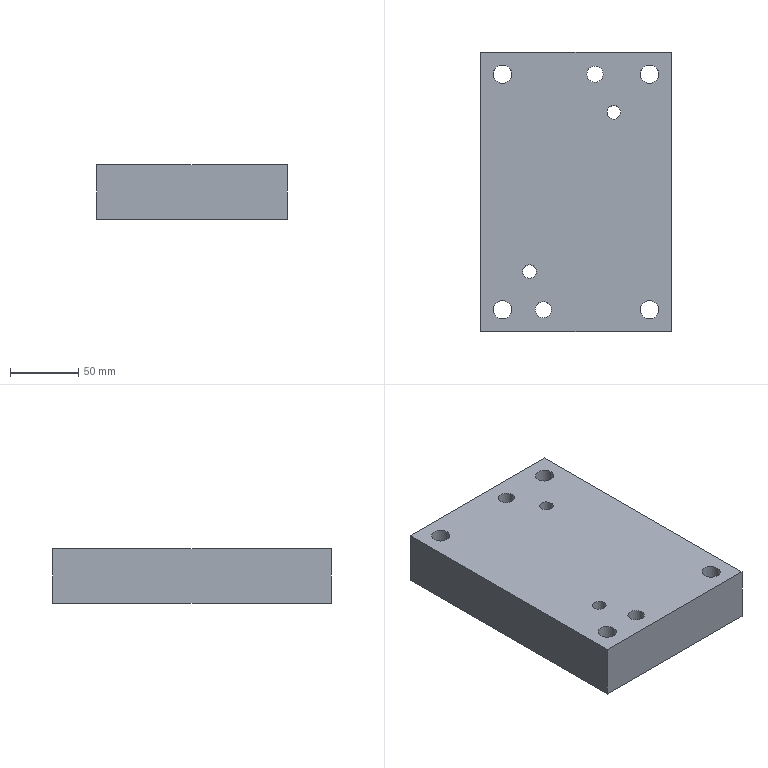Part | STEP file | lll_id762_x_t | 1 solid | 36 faces | box 140 x 205 x 40 mm | volume 1088950 mm3 | cylinder 19 | plane 10 | cone 7 | commonest cylinder face diameters 8.506 x4 13.509 x4 20.007 x4 8.505 x3 10 x2 12 x2
STEP:
#1=CARTESIAN_POINT('',(3881.234,-22.52,102.5));
#2=VERTEX_POINT('',#1);
#3=CARTESIAN_POINT('',(3876.982,-22.52,102.5));
#4=DIRECTION('',(0.,0.,1.));
#5=DIRECTION('',(1.,0.,0.));
#6=AXIS2_PLACEMENT_3D('',#3,#4,#5);
#7=CIRCLE('',#6,4.253);
#8=EDGE_CURVE('',#2,#2,#7,.T.);
#9=ORIENTED_EDGE('',*,*,#8,.T.);
#10=EDGE_LOOP('',(#9));
#11=FACE_BOUND('',#10,.T.);
#12=CARTESIAN_POINT('',(3798.187,86.5,102.5));
#13=VERTEX_POINT('',#12);
#14=CARTESIAN_POINT('',(3788.184,86.5,102.5));
#15=DIRECTION('',(0.,0.,1.));
#16=DIRECTION('',(1.,0.,0.));
#17=AXIS2_PLACEMENT_3D('',#14,#15,#16);
#18=CIRCLE('',#17,10.004);
#19=EDGE_CURVE('',#13,#13,#18,.T.);
#20=ORIENTED_EDGE('',*,*,#19,.T.);
#21=EDGE_LOOP('',(#20));
#22=FACE_BOUND('',#21,.T.);
#23=CARTESIAN_POINT('',(3798.187,-86.5,102.5));
#24=VERTEX_POINT('',#23);
#25=CARTESIAN_POINT('',(3788.184,-86.5,102.5));
#26=DIRECTION('',(0.,0.,1.));
#27=DIRECTION('',(1.,0.,0.));
#28=AXIS2_PLACEMENT_3D('',#25,#26,#27);
#29=CIRCLE('',#28,10.004);
#30=EDGE_CURVE('',#24,#24,#29,.T.);
#31=ORIENTED_EDGE('',*,*,#30,.T.);
#32=EDGE_LOOP('',(#31));
#33=FACE_BOUND('',#32,.T.);
#34=CARTESIAN_POINT('',(3812.184,-86.5,102.5));
#35=VERTEX_POINT('',#34);
#36=CARTESIAN_POINT('',(3818.184,-86.5,102.5));
#37=DIRECTION('',(0.,0.,-1.));
#38=DIRECTION('',(-1.,0.,0.));
#39=AXIS2_PLACEMENT_3D('',#36,#37,#38);
#40=CIRCLE('',#39,6.);
#41=EDGE_CURVE('',#35,#35,#40,.T.);
#42=ORIENTED_EDGE('',*,*,#41,.F.);
#43=EDGE_LOOP('',(#42));
#44=FACE_BOUND('',#43,.T.);
#45=CARTESIAN_POINT('',(3890.747,58.5,102.5));
#46=VERTEX_POINT('',#45);
#47=CARTESIAN_POINT('',(3895.,58.5,102.5));
#48=DIRECTION('',(0.,0.,-1.));
#49=DIRECTION('',(-1.,0.,0.));
#50=AXIS2_PLACEMENT_3D('',#47,#48,#49);
#51=CIRCLE('',#50,4.253);
#52=EDGE_CURVE('',#46,#46,#51,.T.);
#53=ORIENTED_EDGE('',*,*,#52,.F.);
#54=EDGE_LOOP('',(#53));
#55=FACE_BOUND('',#54,.T.);
#56=CARTESIAN_POINT('',(3785.747,-58.5,102.5));
#57=VERTEX_POINT('',#56);
#58=CARTESIAN_POINT('',(3790.,-58.5,102.5));
#59=DIRECTION('',(0.,0.,-1.));
#60=DIRECTION('',(-1.,0.,0.));
#61=AXIS2_PLACEMENT_3D('',#58,#59,#60);
#62=CIRCLE('',#61,4.253);
#63=EDGE_CURVE('',#57,#57,#62,.T.);
#64=ORIENTED_EDGE('',*,*,#63,.F.);
#65=EDGE_LOOP('',(#64));
#66=FACE_BOUND('',#65,.T.);
#67=CARTESIAN_POINT('',(3795.747,58.5,102.5));
#68=VERTEX_POINT('',#67);
#69=CARTESIAN_POINT('',(3800.,58.5,102.5));
#70=DIRECTION('',(0.,0.,-1.));
#71=DIRECTION('',(-1.,0.,0.));
#72=AXIS2_PLACEMENT_3D('',#69,#70,#71);
#73=CIRCLE('',#72,4.253);
#74=EDGE_CURVE('',#68,#68,#73,.T.);
#75=ORIENTED_EDGE('',*,*,#74,.F.);
#76=EDGE_LOOP('',(#75));
#77=FACE_BOUND('',#76,.T.);
#78=CARTESIAN_POINT('',(3890.747,-58.5,102.5));
#79=VERTEX_POINT('',#78);
#80=CARTESIAN_POINT('',(3895.,-58.5,102.5));
#81=DIRECTION('',(0.,0.,-1.));
#82=DIRECTION('',(-1.,0.,0.));
#83=AXIS2_PLACEMENT_3D('',#80,#81,#82);
#84=CIRCLE('',#83,4.253);
#85=EDGE_CURVE('',#79,#79,#84,.T.);
#86=ORIENTED_EDGE('',*,*,#85,.F.);
#87=EDGE_LOOP('',(#86));
#88=FACE_BOUND('',#87,.T.);
#89=CARTESIAN_POINT('',(3803.,-58.5,102.5));
#90=VERTEX_POINT('',#89);
#91=CARTESIAN_POINT('',(3808.,-58.5,102.5));
#92=DIRECTION('',(0.,0.,-1.));
#93=DIRECTION('',(-1.,0.,0.));
#94=AXIS2_PLACEMENT_3D('',#91,#92,#93);
#95=CIRCLE('',#94,5.);
#96=EDGE_CURVE('',#90,#90,#95,.T.);
#97=ORIENTED_EDGE('',*,*,#96,.F.);
#98=EDGE_LOOP('',(#97));
#99=FACE_BOUND('',#98,.T.);
#100=CARTESIAN_POINT('',(3865.,58.5,102.5));
#101=VERTEX_POINT('',#100);
#102=CARTESIAN_POINT('',(3870.,58.5,102.5));
#103=DIRECTION('',(0.,0.,-1.));
#104=DIRECTION('',(-1.,0.,0.));
#105=AXIS2_PLACEMENT_3D('',#102,#103,#104);
#106=CIRCLE('',#105,5.);
#107=EDGE_CURVE('',#101,#101,#106,.T.);
#108=ORIENTED_EDGE('',*,*,#107,.F.);
#109=EDGE_LOOP('',(#108));
#110=FACE_BOUND('',#109,.T.);
#111=CARTESIAN_POINT('',(3772.184,102.5,102.5));
#112=VERTEX_POINT('',#111);
#113=CARTESIAN_POINT('',(3772.184,-102.5,102.5));
#114=VERTEX_POINT('',#113);
#115=CARTESIAN_POINT('',(3772.184,-1.742,102.5));
#116=DIRECTION('',(0.,-1.,0.));
#117=VECTOR('',#116,1.);
#118=LINE('',#115,#117);
#119=EDGE_CURVE('',#112,#114,#118,.T.);
#120=ORIENTED_EDGE('',*,*,#119,.F.);
#121=CARTESIAN_POINT('',(3912.184,102.5,102.5));
#122=VERTEX_POINT('',#121);
#123=CARTESIAN_POINT('',(3532.184,102.5,102.5));
#124=DIRECTION('',(-1.,0.,0.));
#125=VECTOR('',#124,1.);
#126=LINE('',#123,#125);
#127=EDGE_CURVE('',#122,#112,#126,.T.);
#128=ORIENTED_EDGE('',*,*,#127,.F.);
#129=CARTESIAN_POINT('',(3912.184,-102.5,102.5));
#130=VERTEX_POINT('',#129);
#131=CARTESIAN_POINT('',(3912.184,-275.288,102.5));
#132=DIRECTION('',(0.,1.,0.));
#133=VECTOR('',#132,1.);
#134=LINE('',#131,#133);
#135=EDGE_CURVE('',#130,#122,#134,.T.);
#136=ORIENTED_EDGE('',*,*,#135,.F.);
#137=CARTESIAN_POINT('',(3532.184,-102.5,102.5));
#138=DIRECTION('',(-1.,0.,0.));
#139=VECTOR('',#138,1.);
#140=LINE('',#137,#139);
#141=EDGE_CURVE('',#130,#114,#140,.T.);
#142=ORIENTED_EDGE('',*,*,#141,.T.);
#143=EDGE_LOOP('',(#120,#128,#136,#142));
#144=FACE_BOUND('',#143,.T.);
#145=CARTESIAN_POINT('',(3906.187,-86.5,102.5));
#146=VERTEX_POINT('',#145);
#147=CARTESIAN_POINT('',(3896.184,-86.5,102.5));
#148=DIRECTION('',(0.,0.,1.));
#149=DIRECTION('',(1.,0.,0.));
#150=AXIS2_PLACEMENT_3D('',#147,#148,#149);
#151=CIRCLE('',#150,10.004);
#152=EDGE_CURVE('',#146,#146,#151,.T.);
#153=ORIENTED_EDGE('',*,*,#152,.T.);
#154=EDGE_LOOP('',(#153));
#155=FACE_BOUND('',#154,.T.);
#156=CARTESIAN_POINT('',(3850.184,86.5,102.5));
#157=VERTEX_POINT('',#156);
#158=CARTESIAN_POINT('',(3856.184,86.5,102.5));
#159=DIRECTION('',(0.,0.,-1.));
#160=DIRECTION('',(-1.,0.,0.));
#161=AXIS2_PLACEMENT_3D('',#158,#159,#160);
#162=CIRCLE('',#161,6.);
#163=EDGE_CURVE('',#157,#157,#162,.T.);
#164=ORIENTED_EDGE('',*,*,#163,.F.);
#165=EDGE_LOOP('',(#164));
#166=FACE_BOUND('',#165,.T.);
#167=CARTESIAN_POINT('',(3906.187,86.5,102.5));
#168=VERTEX_POINT('',#167);
#169=CARTESIAN_POINT('',(3896.184,86.5,102.5));
#170=DIRECTION('',(0.,0.,1.));
#171=DIRECTION('',(1.,0.,0.));
#172=AXIS2_PLACEMENT_3D('',#169,#170,#171);
#173=CIRCLE('',#172,10.004);
#174=EDGE_CURVE('',#168,#168,#173,.T.);
#175=ORIENTED_EDGE('',*,*,#174,.T.);
#176=EDGE_LOOP('',(#175));
#177=FACE_BOUND('',#176,.T.);
#178=CARTESIAN_POINT('',(3843.234,-0.01982,102.5));
#179=VERTEX_POINT('',#178);
#180=CARTESIAN_POINT('',(3838.982,-0.01982,102.5));
#181=DIRECTION('',(0.,0.,1.));
#182=DIRECTION('',(1.,0.,0.));
#183=AXIS2_PLACEMENT_3D('',#180,#181,#182);
#184=CIRCLE('',#183,4.253);
#185=EDGE_CURVE('',#179,#179,#184,.T.);
#186=ORIENTED_EDGE('',*,*,#185,.T.);
#187=EDGE_LOOP('',(#186));
#188=FACE_BOUND('',#187,.T.);
#189=CARTESIAN_POINT('',(3881.252,22.5,102.5));
#190=VERTEX_POINT('',#189);
#191=CARTESIAN_POINT('',(3877.,22.5,102.5));
#192=DIRECTION('',(0.,0.,1.));
#193=DIRECTION('',(1.,0.,0.));
#194=AXIS2_PLACEMENT_3D('',#191,#192,#193);
#195=CIRCLE('',#194,4.253);
#196=EDGE_CURVE('',#190,#190,#195,.T.);
#197=ORIENTED_EDGE('',*,*,#196,.T.);
#198=EDGE_LOOP('',(#197));
#199=FACE_BOUND('',#198,.T.);
#200=CARTESIAN_POINT('',(3532.184,-1.742,102.5));
#201=DIRECTION('',(0.,0.,-1.));
#202=DIRECTION('',(-1.,0.,0.));
#203=AXIS2_PLACEMENT_3D('',#200,#201,#202);
#204=PLANE('',#203);
#205=ADVANCED_FACE('',(#11,#22,#33,#44,#55,#66,#77,#88,#99,#110,#144,#155,#166,#177,#188,#199),#204,.T.);
#206=CARTESIAN_POINT('',(3794.938,86.5,142.5));
#207=VERTEX_POINT('',#206);
#208=CARTESIAN_POINT('',(3788.184,86.5,142.5));
#209=DIRECTION('',(0.,0.,1.));
#210=DIRECTION('',(1.,0.,0.));
#211=AXIS2_PLACEMENT_3D('',#208,#209,#210);
#212=CIRCLE('',#211,6.755);
#213=EDGE_CURVE('',#207,#207,#212,.T.);
#214=ORIENTED_EDGE('',*,*,#213,.F.);
#215=EDGE_LOOP('',(#214));
#216=FACE_BOUND('',#215,.T.);
#217=CARTESIAN_POINT('',(3902.938,86.5,142.5));
#218=VERTEX_POINT('',#217);
#219=CARTESIAN_POINT('',(3896.184,86.5,142.5));
#220=DIRECTION('',(0.,0.,1.));
#221=DIRECTION('',(1.,0.,0.));
#222=AXIS2_PLACEMENT_3D('',#219,#220,#221);
#223=CIRCLE('',#222,6.755);
#224=EDGE_CURVE('',#218,#218,#223,.T.);
#225=ORIENTED_EDGE('',*,*,#224,.F.);
#226=EDGE_LOOP('',(#225));
#227=FACE_BOUND('',#226,.T.);
#228=CARTESIAN_POINT('',(3862.184,86.5,142.5));
#229=VERTEX_POINT('',#228);
#230=CARTESIAN_POINT('',(3856.184,86.5,142.5));
#231=DIRECTION('',(0.,0.,1.));
#232=DIRECTION('',(1.,0.,0.));
#233=AXIS2_PLACEMENT_3D('',#230,#231,#232);
#234=CIRCLE('',#233,6.);
#235=EDGE_CURVE('',#229,#229,#234,.T.);
#236=ORIENTED_EDGE('',*,*,#235,.F.);
#237=EDGE_LOOP('',(#236));
#238=FACE_BOUND('',#237,.T.);
#239=CARTESIAN_POINT('',(3794.938,-86.5,142.5));
#240=VERTEX_POINT('',#239);
#241=CARTESIAN_POINT('',(3788.184,-86.5,142.5));
#242=DIRECTION('',(0.,0.,1.));
#243=DIRECTION('',(1.,0.,0.));
#244=AXIS2_PLACEMENT_3D('',#241,#242,#243);
#245=CIRCLE('',#244,6.755);
#246=EDGE_CURVE('',#240,#240,#245,.T.);
#247=ORIENTED_EDGE('',*,*,#246,.F.);
#248=EDGE_LOOP('',(#247));
#249=FACE_BOUND('',#248,.T.);
#250=CARTESIAN_POINT('',(3824.184,-86.5,142.5));
#251=VERTEX_POINT('',#250);
#252=CARTESIAN_POINT('',(3818.184,-86.5,142.5));
#253=DIRECTION('',(0.,0.,1.));
#254=DIRECTION('',(1.,0.,0.));
#255=AXIS2_PLACEMENT_3D('',#252,#253,#254);
#256=CIRCLE('',#255,6.);
#257=EDGE_CURVE('',#251,#251,#256,.T.);
#258=ORIENTED_EDGE('',*,*,#257,.F.);
#259=EDGE_LOOP('',(#258));
#260=FACE_BOUND('',#259,.T.);
#261=CARTESIAN_POINT('',(3902.938,-86.5,142.5));
#262=VERTEX_POINT('',#261);
#263=CARTESIAN_POINT('',(3896.184,-86.5,142.5));
#264=DIRECTION('',(0.,0.,1.));
#265=DIRECTION('',(1.,0.,0.));
#266=AXIS2_PLACEMENT_3D('',#263,#264,#265);
#267=CIRCLE('',#266,6.755);
#268=EDGE_CURVE('',#262,#262,#267,.T.);
#269=ORIENTED_EDGE('',*,*,#268,.F.);
#270=EDGE_LOOP('',(#269));
#271=FACE_BOUND('',#270,.T.);
#272=CARTESIAN_POINT('',(3772.184,102.5,142.5));
#273=VERTEX_POINT('',#272);
#274=CARTESIAN_POINT('',(3772.184,-102.5,142.5));
#275=VERTEX_POINT('',#274);
#276=CARTESIAN_POINT('',(3772.184,0.00007613,142.5));
#277=DIRECTION('',(0.,-1.,0.));
#278=VECTOR('',#277,1.);
#279=LINE('',#276,#278);
#280=EDGE_CURVE('',#273,#275,#279,.T.);
#281=ORIENTED_EDGE('',*,*,#280,.T.);
#282=CARTESIAN_POINT('',(3912.184,-102.5,142.5));
#283=VERTEX_POINT('',#282);
#284=CARTESIAN_POINT('',(3532.184,-102.5,142.5));
#285=DIRECTION('',(1.,0.,0.));
#286=VECTOR('',#285,1.);
#287=LINE('',#284,#286);
#288=EDGE_CURVE('',#275,#283,#287,.T.);
#289=ORIENTED_EDGE('',*,*,#288,.T.);
#290=CARTESIAN_POINT('',(3912.184,102.5,142.5));
#291=VERTEX_POINT('',#290);
#292=CARTESIAN_POINT('',(3912.184,-275.288,142.5));
#293=DIRECTION('',(0.,-1.,0.));
#294=VECTOR('',#293,1.);
#295=LINE('',#292,#294);
#296=EDGE_CURVE('',#291,#283,#295,.T.);
#297=ORIENTED_EDGE('',*,*,#296,.F.);
#298=CARTESIAN_POINT('',(3532.184,102.5,142.5));
#299=DIRECTION('',(1.,0.,0.));
#300=VECTOR('',#299,1.);
#301=LINE('',#298,#300);
#302=EDGE_CURVE('',#273,#291,#301,.T.);
#303=ORIENTED_EDGE('',*,*,#302,.F.);
#304=EDGE_LOOP('',(#281,#289,#297,#303));
#305=FACE_BOUND('',#304,.T.);
#306=CARTESIAN_POINT('',(3875.,58.5,142.5));
#307=VERTEX_POINT('',#306);
#308=CARTESIAN_POINT('',(3870.,58.5,142.5));
#309=DIRECTION('',(0.,0.,1.));
#310=DIRECTION('',(1.,0.,0.));
#311=AXIS2_PLACEMENT_3D('',#308,#309,#310);
#312=CIRCLE('',#311,5.);
#313=EDGE_CURVE('',#307,#307,#312,.T.);
#314=ORIENTED_EDGE('',*,*,#313,.F.);
#315=EDGE_LOOP('',(#314));
#316=FACE_BOUND('',#315,.T.);
#317=CARTESIAN_POINT('',(3813.,-58.5,142.5));
#318=VERTEX_POINT('',#317);
#319=CARTESIAN_POINT('',(3808.,-58.5,142.5));
#320=DIRECTION('',(0.,0.,1.));
#321=DIRECTION('',(1.,0.,0.));
#322=AXIS2_PLACEMENT_3D('',#319,#320,#321);
#323=CIRCLE('',#322,5.);
#324=EDGE_CURVE('',#318,#318,#323,.T.);
#325=ORIENTED_EDGE('',*,*,#324,.F.);
#326=EDGE_LOOP('',(#325));
#327=FACE_BOUND('',#326,.T.);
#328=CARTESIAN_POINT('',(3532.184,-1.742,142.5));
#329=DIRECTION('',(0.,0.,1.));
#330=DIRECTION('',(1.,0.,0.));
#331=AXIS2_PLACEMENT_3D('',#328,#329,#330);
#332=PLANE('',#331);
#333=ADVANCED_FACE('',(#216,#227,#238,#249,#260,#271,#305,#316,#327),#332,.T.);
#334=ORIENTED_EDGE('',*,*,#296,.T.);
#335=CARTESIAN_POINT('',(3912.184,-102.5,102.5));
#336=DIRECTION('',(0.,0.,-1.));
#337=VECTOR('',#336,1.);
#338=LINE('',#335,#337);
#339=EDGE_CURVE('',#283,#130,#338,.T.);
#340=ORIENTED_EDGE('',*,*,#339,.T.);
#341=ORIENTED_EDGE('',*,*,#135,.T.);
#342=CARTESIAN_POINT('',(3912.184,102.5,102.5));
#343=DIRECTION('',(0.,0.,1.));
#344=VECTOR('',#343,1.);
#345=LINE('',#342,#344);
#346=EDGE_CURVE('',#122,#291,#345,.T.);
#347=ORIENTED_EDGE('',*,*,#346,.T.);
#348=EDGE_LOOP('',(#334,#340,#341,#347));
#349=FACE_OUTER_BOUND('',#348,.T.);
#350=CARTESIAN_POINT('',(3912.184,-275.288,102.5));
#351=DIRECTION('',(1.,0.,0.));
#352=DIRECTION('',(0.,0.,-1.));
#353=AXIS2_PLACEMENT_3D('',#350,#351,#352);
#354=PLANE('',#353);
#355=ADVANCED_FACE('',(#349),#354,.T.);
#356=ORIENTED_EDGE('',*,*,#52,.T.);
#357=EDGE_LOOP('',(#356));
#358=FACE_BOUND('',#357,.T.);
#359=CARTESIAN_POINT('',(3899.253,58.5,123.253));
#360=VERTEX_POINT('',#359);
#361=CARTESIAN_POINT('',(3895.,58.5,123.253));
#362=DIRECTION('',(0.,0.,1.));
#363=DIRECTION('',(1.,0.,0.));
#364=AXIS2_PLACEMENT_3D('',#361,#362,#363);
#365=CIRCLE('',#364,4.253);
#366=EDGE_CURVE('',#360,#360,#365,.T.);
#367=ORIENTED_EDGE('',*,*,#366,.T.);
#368=EDGE_LOOP('',(#367));
#369=FACE_BOUND('',#368,.T.);
#370=CARTESIAN_POINT('',(3895.,58.5,92.5));
#371=DIRECTION('',(0.,0.,1.));
#372=DIRECTION('',(-1.,0.,0.));
#373=AXIS2_PLACEMENT_3D('',#370,#371,#372);
#374=CYLINDRICAL_SURFACE('',#373,4.253);
#375=ADVANCED_FACE('',(#358,#369),#374,.F.);
#376=CARTESIAN_POINT('',(3895.,58.5,127.506));
#377=VERTEX_POINT('',#376);
#378=VERTEX_LOOP('',#377);
#379=FACE_BOUND('',#378,.T.);
#380=ORIENTED_EDGE('',*,*,#366,.F.);
#381=EDGE_LOOP('',(#380));
#382=FACE_BOUND('',#381,.T.);
#383=CARTESIAN_POINT('',(3895.,58.5,123.253));
#384=DIRECTION('',(0.,0.,-1.));
#385=DIRECTION('',(1.,0.,0.));
#386=AXIS2_PLACEMENT_3D('',#383,#384,#385);
#387=CONICAL_SURFACE('',#386,4.253,45.);
#388=ADVANCED_FACE('',(#379,#382),#387,.F.);
#389=ORIENTED_EDGE('',*,*,#63,.T.);
#390=EDGE_LOOP('',(#389));
#391=FACE_BOUND('',#390,.T.);
#392=CARTESIAN_POINT('',(3794.253,-58.5,123.253));
#393=VERTEX_POINT('',#392);
#394=CARTESIAN_POINT('',(3790.,-58.5,123.253));
#395=DIRECTION('',(0.,0.,1.));
#396=DIRECTION('',(1.,0.,0.));
#397=AXIS2_PLACEMENT_3D('',#394,#395,#396);
#398=CIRCLE('',#397,4.253);
#399=EDGE_CURVE('',#393,#393,#398,.T.);
#400=ORIENTED_EDGE('',*,*,#399,.T.);
#401=EDGE_LOOP('',(#400));
#402=FACE_BOUND('',#401,.T.);
#403=CARTESIAN_POINT('',(3790.,-58.5,92.5));
#404=DIRECTION('',(0.,0.,1.));
#405=DIRECTION('',(-1.,0.,0.));
#406=AXIS2_PLACEMENT_3D('',#403,#404,#405);
#407=CYLINDRICAL_SURFACE('',#406,4.253);
#408=ADVANCED_FACE('',(#391,#402),#407,.F.);
#409=CARTESIAN_POINT('',(3790.,-58.5,127.506));
#410=VERTEX_POINT('',#409);
#411=VERTEX_LOOP('',#410);
#412=FACE_BOUND('',#411,.T.);
#413=ORIENTED_EDGE('',*,*,#399,.F.);
#414=EDGE_LOOP('',(#413));
#415=FACE_BOUND('',#414,.T.);
#416=CARTESIAN_POINT('',(3790.,-58.5,123.253));
#417=DIRECTION('',(0.,0.,-1.));
#418=DIRECTION('',(1.,0.,0.));
#419=AXIS2_PLACEMENT_3D('',#416,#417,#418);
#420=CONICAL_SURFACE('',#419,4.253,45.);
#421=ADVANCED_FACE('',(#412,#415),#420,.F.);
#422=ORIENTED_EDGE('',*,*,#74,.T.);
#423=EDGE_LOOP('',(#422));
#424=FACE_BOUND('',#423,.T.);
#425=CARTESIAN_POINT('',(3804.253,58.5,123.253));
#426=VERTEX_POINT('',#425);
#427=CARTESIAN_POINT('',(3800.,58.5,123.253));
#428=DIRECTION('',(0.,0.,1.));
#429=DIRECTION('',(1.,0.,0.));
#430=AXIS2_PLACEMENT_3D('',#427,#428,#429);
#431=CIRCLE('',#430,4.253);
#432=EDGE_CURVE('',#426,#426,#431,.T.);
#433=ORIENTED_EDGE('',*,*,#432,.T.);
#434=EDGE_LOOP('',(#433));
#435=FACE_BOUND('',#434,.T.);
#436=CARTESIAN_POINT('',(3800.,58.5,92.5));
#437=DIRECTION('',(0.,0.,1.));
#438=DIRECTION('',(-1.,0.,0.));
#439=AXIS2_PLACEMENT_3D('',#436,#437,#438);
#440=CYLINDRICAL_SURFACE('',#439,4.253);
#441=ADVANCED_FACE('',(#424,#435),#440,.F.);
#442=CARTESIAN_POINT('',(3800.,58.5,127.506));
#443=VERTEX_POINT('',#442);
#444=VERTEX_LOOP('',#443);
#445=FACE_BOUND('',#444,.T.);
#446=ORIENTED_EDGE('',*,*,#432,.F.);
#447=EDGE_LOOP('',(#446));
#448=FACE_BOUND('',#447,.T.);
#449=CARTESIAN_POINT('',(3800.,58.5,123.253));
#450=DIRECTION('',(0.,0.,-1.));
#451=DIRECTION('',(1.,0.,0.));
#452=AXIS2_PLACEMENT_3D('',#449,#450,#451);
#453=CONICAL_SURFACE('',#452,4.253,45.);
#454=ADVANCED_FACE('',(#445,#448),#453,.F.);
#455=ORIENTED_EDGE('',*,*,#85,.T.);
#456=EDGE_LOOP('',(#455));
#457=FACE_BOUND('',#456,.T.);
#458=CARTESIAN_POINT('',(3899.253,-58.5,123.253));
#459=VERTEX_POINT('',#458);
#460=CARTESIAN_POINT('',(3895.,-58.5,123.253));
#461=DIRECTION('',(0.,0.,1.));
#462=DIRECTION('',(1.,0.,0.));
#463=AXIS2_PLACEMENT_3D('',#460,#461,#462);
#464=CIRCLE('',#463,4.253);
#465=EDGE_CURVE('',#459,#459,#464,.T.);
#466=ORIENTED_EDGE('',*,*,#465,.T.);
#467=EDGE_LOOP('',(#466));
#468=FACE_BOUND('',#467,.T.);
#469=CARTESIAN_POINT('',(3895.,-58.5,92.5));
#470=DIRECTION('',(0.,0.,1.));
#471=DIRECTION('',(-1.,0.,0.));
#472=AXIS2_PLACEMENT_3D('',#469,#470,#471);
#473=CYLINDRICAL_SURFACE('',#472,4.253);
#474=ADVANCED_FACE('',(#457,#468),#473,.F.);
#475=CARTESIAN_POINT('',(3895.,-58.5,127.506));
#476=VERTEX_POINT('',#475);
#477=VERTEX_LOOP('',#476);
#478=FACE_BOUND('',#477,.T.);
#479=ORIENTED_EDGE('',*,*,#465,.F.);
#480=EDGE_LOOP('',(#479));
#481=FACE_BOUND('',#480,.T.);
#482=CARTESIAN_POINT('',(3895.,-58.5,123.253));
#483=DIRECTION('',(0.,0.,-1.));
#484=DIRECTION('',(1.,0.,0.));
#485=AXIS2_PLACEMENT_3D('',#482,#483,#484);
#486=CONICAL_SURFACE('',#485,4.253,45.);
#487=ADVANCED_FACE('',(#478,#481),#486,.F.);
#488=ORIENTED_EDGE('',*,*,#96,.T.);
#489=EDGE_LOOP('',(#488));
#490=FACE_BOUND('',#489,.T.);
#491=ORIENTED_EDGE('',*,*,#324,.T.);
#492=EDGE_LOOP('',(#491));
#493=FACE_BOUND('',#492,.T.);
#494=CARTESIAN_POINT('',(3808.,-58.5,60.5));
#495=DIRECTION('',(0.,0.,1.));
#496=DIRECTION('',(-1.,0.,0.));
#497=AXIS2_PLACEMENT_3D('',#494,#495,#496);
#498=CYLINDRICAL_SURFACE('',#497,5.);
#499=ADVANCED_FACE('',(#490,#493),#498,.F.);
#500=ORIENTED_EDGE('',*,*,#107,.T.);
#501=EDGE_LOOP('',(#500));
#502=FACE_BOUND('',#501,.T.);
#503=ORIENTED_EDGE('',*,*,#313,.T.);
#504=EDGE_LOOP('',(#503));
#505=FACE_BOUND('',#504,.T.);
#506=CARTESIAN_POINT('',(3870.,58.5,60.5));
#507=DIRECTION('',(0.,0.,1.));
#508=DIRECTION('',(-1.,0.,0.));
#509=AXIS2_PLACEMENT_3D('',#506,#507,#508);
#510=CYLINDRICAL_SURFACE('',#509,5.);
#511=ADVANCED_FACE('',(#502,#505),#510,.F.);
#512=CARTESIAN_POINT('',(3772.184,102.5,76.5));
#513=DIRECTION('',(0.,0.,-1.));
#514=VECTOR('',#513,1.);
#515=LINE('',#512,#514);
#516=EDGE_CURVE('',#273,#112,#515,.T.);
#517=ORIENTED_EDGE('',*,*,#516,.F.);
#518=ORIENTED_EDGE('',*,*,#302,.T.);
#519=ORIENTED_EDGE('',*,*,#346,.F.);
#520=ORIENTED_EDGE('',*,*,#127,.T.);
#521=EDGE_LOOP('',(#517,#518,#519,#520));
#522=FACE_OUTER_BOUND('',#521,.T.);
#523=CARTESIAN_POINT('',(3842.5,102.5,76.5));
#524=DIRECTION('',(0.,1.,0.));
#525=DIRECTION('',(0.,0.,-1.));
#526=AXIS2_PLACEMENT_3D('',#523,#524,#525);
#527=PLANE('',#526);
#528=ADVANCED_FACE('',(#522),#527,.T.);
#529=CARTESIAN_POINT('',(3772.184,-102.5,76.5));
#530=DIRECTION('',(0.,0.,1.));
#531=VECTOR('',#530,1.);
#532=LINE('',#529,#531);
#533=EDGE_CURVE('',#114,#275,#532,.T.);
#534=ORIENTED_EDGE('',*,*,#533,.F.);
#535=ORIENTED_EDGE('',*,*,#141,.F.);
#536=ORIENTED_EDGE('',*,*,#339,.F.);
#537=ORIENTED_EDGE('',*,*,#288,.F.);
#538=EDGE_LOOP('',(#534,#535,#536,#537));
#539=FACE_OUTER_BOUND('',#538,.T.);
#540=CARTESIAN_POINT('',(3842.5,-102.5,76.5));
#541=DIRECTION('',(0.,-1.,0.));
#542=DIRECTION('',(0.,0.,1.));
#543=AXIS2_PLACEMENT_3D('',#540,#541,#542);
#544=PLANE('',#543);
#545=ADVANCED_FACE('',(#539),#544,.T.);
#546=ORIENTED_EDGE('',*,*,#516,.T.);
#547=ORIENTED_EDGE('',*,*,#119,.T.);
#548=ORIENTED_EDGE('',*,*,#533,.T.);
#549=ORIENTED_EDGE('',*,*,#280,.F.);
#550=EDGE_LOOP('',(#546,#547,#548,#549));
#551=FACE_OUTER_BOUND('',#550,.T.);
#552=CARTESIAN_POINT('',(3772.184,0.00007613,122.5));
#553=DIRECTION('',(1.,0.,0.));
#554=DIRECTION('',(0.,0.,1.));
#555=AXIS2_PLACEMENT_3D('',#552,#553,#554);
#556=PLANE('',#555);
#557=ADVANCED_FACE('',(#551),#556,.F.);
#558=ORIENTED_EDGE('',*,*,#268,.T.);
#559=EDGE_LOOP('',(#558));
#560=FACE_BOUND('',#559,.T.);
#561=CARTESIAN_POINT('',(3902.938,-86.5,117.5));
#562=VERTEX_POINT('',#561);
#563=CARTESIAN_POINT('',(3896.184,-86.5,117.5));
#564=DIRECTION('',(0.,0.,1.));
#565=DIRECTION('',(1.,0.,0.));
#566=AXIS2_PLACEMENT_3D('',#563,#564,#565);
#567=CIRCLE('',#566,6.755);
#568=EDGE_CURVE('',#562,#562,#567,.T.);
#569=ORIENTED_EDGE('',*,*,#568,.F.);
#570=EDGE_LOOP('',(#569));
#571=FACE_BOUND('',#570,.T.);
#572=CARTESIAN_POINT('',(3896.184,-86.5,97.5));
#573=DIRECTION('',(0.,0.,1.));
#574=DIRECTION('',(-1.,0.,0.));
#575=AXIS2_PLACEMENT_3D('',#572,#573,#574);
#576=CYLINDRICAL_SURFACE('',#575,6.755);
#577=ADVANCED_FACE('',(#560,#571),#576,.F.);
#578=ORIENTED_EDGE('',*,*,#568,.T.);
#579=EDGE_LOOP('',(#578));
#580=FACE_BOUND('',#579,.T.);
#581=CARTESIAN_POINT('',(3906.187,-86.5,117.5));
#582=VERTEX_POINT('',#581);
#583=CARTESIAN_POINT('',(3896.184,-86.5,117.5));
#584=DIRECTION('',(0.,0.,1.));
#585=DIRECTION('',(1.,0.,0.));
#586=AXIS2_PLACEMENT_3D('',#583,#584,#585);
#587=CIRCLE('',#586,10.004);
#588=EDGE_CURVE('',#582,#582,#587,.T.);
#589=ORIENTED_EDGE('',*,*,#588,.F.);
#590=EDGE_LOOP('',(#589));
#591=FACE_BOUND('',#590,.T.);
#592=CARTESIAN_POINT('',(3896.184,-86.5,117.5));
#593=DIRECTION('',(0.,0.,1.));
#594=DIRECTION('',(-1.,0.,0.));
#595=AXIS2_PLACEMENT_3D('',#592,#593,#594);
#596=PLANE('',#595);
#597=ADVANCED_FACE('',(#580,#591),#596,.F.);
#598=ORIENTED_EDGE('',*,*,#588,.T.);
#599=EDGE_LOOP('',(#598));
#600=FACE_BOUND('',#599,.T.);
#601=ORIENTED_EDGE('',*,*,#152,.F.);
#602=EDGE_LOOP('',(#601));
#603=FACE_BOUND('',#602,.T.);
#604=CARTESIAN_POINT('',(3896.184,-86.5,102.5));
#605=DIRECTION('',(0.,0.,1.));
#606=DIRECTION('',(-1.,0.,0.));
#607=AXIS2_PLACEMENT_3D('',#604,#605,#606);
#608=CYLINDRICAL_SURFACE('',#607,10.004);
#609=ADVANCED_FACE('',(#600,#603),#608,.F.);
#610=ORIENTED_EDGE('',*,*,#41,.T.);
#611=EDGE_LOOP('',(#610));
#612=FACE_BOUND('',#611,.T.);
#613=ORIENTED_EDGE('',*,*,#257,.T.);
#614=EDGE_LOOP('',(#613));
#615=FACE_BOUND('',#614,.T.);
#616=CARTESIAN_POINT('',(3818.184,-86.5,97.5));
#617=DIRECTION('',(0.,0.,1.));
#618=DIRECTION('',(-1.,0.,0.));
#619=AXIS2_PLACEMENT_3D('',#616,#617,#618);
#620=CYLINDRICAL_SURFACE('',#619,6.);
#621=ADVANCED_FACE('',(#612,#615),#620,.F.);
#622=ORIENTED_EDGE('',*,*,#246,.T.);
#623=EDGE_LOOP('',(#622));
#624=FACE_BOUND('',#623,.T.);
#625=CARTESIAN_POINT('',(3794.938,-86.5,117.5));
#626=VERTEX_POINT('',#625);
#627=CARTESIAN_POINT('',(3788.184,-86.5,117.5));
#628=DIRECTION('',(0.,0.,1.));
#629=DIRECTION('',(1.,0.,0.));
#630=AXIS2_PLACEMENT_3D('',#627,#628,#629);
#631=CIRCLE('',#630,6.755);
#632=EDGE_CURVE('',#626,#626,#631,.T.);
#633=ORIENTED_EDGE('',*,*,#632,.F.);
#634=EDGE_LOOP('',(#633));
#635=FACE_BOUND('',#634,.T.);
#636=CARTESIAN_POINT('',(3788.184,-86.5,97.5));
#637=DIRECTION('',(0.,0.,1.));
#638=DIRECTION('',(-1.,0.,0.));
#639=AXIS2_PLACEMENT_3D('',#636,#637,#638);
#640=CYLINDRICAL_SURFACE('',#639,6.755);
#641=ADVANCED_FACE('',(#624,#635),#640,.F.);
#642=ORIENTED_EDGE('',*,*,#632,.T.);
#643=EDGE_LOOP('',(#642));
#644=FACE_BOUND('',#643,.T.);
#645=CARTESIAN_POINT('',(3798.187,-86.5,117.5));
#646=VERTEX_POINT('',#645);
#647=CARTESIAN_POINT('',(3788.184,-86.5,117.5));
#648=DIRECTION('',(0.,0.,1.));
#649=DIRECTION('',(1.,0.,0.));
#650=AXIS2_PLACEMENT_3D('',#647,#648,#649);
#651=CIRCLE('',#650,10.004);
#652=EDGE_CURVE('',#646,#646,#651,.T.);
#653=ORIENTED_EDGE('',*,*,#652,.F.);
#654=EDGE_LOOP('',(#653));
#655=FACE_BOUND('',#654,.T.);
#656=CARTESIAN_POINT('',(3788.184,-86.5,117.5));
#657=DIRECTION('',(0.,0.,1.));
#658=DIRECTION('',(-1.,0.,0.));
#659=AXIS2_PLACEMENT_3D('',#656,#657,#658);
#660=PLANE('',#659);
#661=ADVANCED_FACE('',(#644,#655),#660,.F.);
#662=ORIENTED_EDGE('',*,*,#652,.T.);
#663=EDGE_LOOP('',(#662));
#664=FACE_BOUND('',#663,.T.);
#665=ORIENTED_EDGE('',*,*,#30,.F.);
#666=EDGE_LOOP('',(#665));
#667=FACE_BOUND('',#666,.T.);
#668=CARTESIAN_POINT('',(3788.184,-86.5,102.5));
#669=DIRECTION('',(0.,0.,1.));
#670=DIRECTION('',(-1.,0.,0.));
#671=AXIS2_PLACEMENT_3D('',#668,#669,#670);
#672=CYLINDRICAL_SURFACE('',#671,10.004);
#673=ADVANCED_FACE('',(#664,#667),#672,.F.);
#674=ORIENTED_EDGE('',*,*,#163,.T.);
#675=EDGE_LOOP('',(#674));
#676=FACE_BOUND('',#675,.T.);
#677=ORIENTED_EDGE('',*,*,#235,.T.);
#678=EDGE_LOOP('',(#677));
#679=FACE_BOUND('',#678,.T.);
#680=CARTESIAN_POINT('',(3856.184,86.5,97.5));
#681=DIRECTION('',(0.,0.,1.));
#682=DIRECTION('',(-1.,0.,0.));
#683=AXIS2_PLACEMENT_3D('',#680,#681,#682);
#684=CYLINDRICAL_SURFACE('',#683,6.);
#685=ADVANCED_FACE('',(#676,#679),#684,.F.);
#686=ORIENTED_EDGE('',*,*,#224,.T.);
#687=EDGE_LOOP('',(#686));
#688=FACE_BOUND('',#687,.T.);
#689=CARTESIAN_POINT('',(3902.938,86.5,117.5));
#690=VERTEX_POINT('',#689);
#691=CARTESIAN_POINT('',(3896.184,86.5,117.5));
#692=DIRECTION('',(0.,0.,1.));
#693=DIRECTION('',(1.,0.,0.));
#694=AXIS2_PLACEMENT_3D('',#691,#692,#693);
#695=CIRCLE('',#694,6.755);
#696=EDGE_CURVE('',#690,#690,#695,.T.);
#697=ORIENTED_EDGE('',*,*,#696,.F.);
#698=EDGE_LOOP('',(#697));
#699=FACE_BOUND('',#698,.T.);
#700=CARTESIAN_POINT('',(3896.184,86.5,97.5));
#701=DIRECTION('',(0.,0.,1.));
#702=DIRECTION('',(-1.,0.,0.));
#703=AXIS2_PLACEMENT_3D('',#700,#701,#702);
#704=CYLINDRICAL_SURFACE('',#703,6.755);
#705=ADVANCED_FACE('',(#688,#699),#704,.F.);
#706=ORIENTED_EDGE('',*,*,#696,.T.);
#707=EDGE_LOOP('',(#706));
#708=FACE_BOUND('',#707,.T.);
#709=CARTESIAN_POINT('',(3906.187,86.5,117.5));
#710=VERTEX_POINT('',#709);
#711=CARTESIAN_POINT('',(3896.184,86.5,117.5));
#712=DIRECTION('',(0.,0.,1.));
#713=DIRECTION('',(1.,0.,0.));
#714=AXIS2_PLACEMENT_3D('',#711,#712,#713);
#715=CIRCLE('',#714,10.004);
#716=EDGE_CURVE('',#710,#710,#715,.T.);
#717=ORIENTED_EDGE('',*,*,#716,.F.);
#718=EDGE_LOOP('',(#717));
#719=FACE_BOUND('',#718,.T.);
#720=CARTESIAN_POINT('',(3896.184,86.5,117.5));
#721=DIRECTION('',(0.,0.,1.));
#722=DIRECTION('',(-1.,0.,0.));
#723=AXIS2_PLACEMENT_3D('',#720,#721,#722);
#724=PLANE('',#723);
#725=ADVANCED_FACE('',(#708,#719),#724,.F.);
#726=ORIENTED_EDGE('',*,*,#716,.T.);
#727=EDGE_LOOP('',(#726));
#728=FACE_BOUND('',#727,.T.);
#729=ORIENTED_EDGE('',*,*,#174,.F.);
#730=EDGE_LOOP('',(#729));
#731=FACE_BOUND('',#730,.T.);
#732=CARTESIAN_POINT('',(3896.184,86.5,102.5));
#733=DIRECTION('',(0.,0.,1.));
#734=DIRECTION('',(-1.,0.,0.));
#735=AXIS2_PLACEMENT_3D('',#732,#733,#734);
#736=CYLINDRICAL_SURFACE('',#735,10.004);
#737=ADVANCED_FACE('',(#728,#731),#736,.F.);
#738=ORIENTED_EDGE('',*,*,#213,.T.);
#739=EDGE_LOOP('',(#738));
#740=FACE_BOUND('',#739,.T.);
#741=CARTESIAN_POINT('',(3794.938,86.5,117.5));
#742=VERTEX_POINT('',#741);
#743=CARTESIAN_POINT('',(3788.184,86.5,117.5));
#744=DIRECTION('',(0.,0.,1.));
#745=DIRECTION('',(1.,0.,0.));
#746=AXIS2_PLACEMENT_3D('',#743,#744,#745);
#747=CIRCLE('',#746,6.755);
#748=EDGE_CURVE('',#742,#742,#747,.T.);
#749=ORIENTED_EDGE('',*,*,#748,.F.);
#750=EDGE_LOOP('',(#749));
#751=FACE_BOUND('',#750,.T.);
#752=CARTESIAN_POINT('',(3788.184,86.5,97.5));
#753=DIRECTION('',(0.,0.,1.));
#754=DIRECTION('',(-1.,0.,0.));
#755=AXIS2_PLACEMENT_3D('',#752,#753,#754);
#756=CYLINDRICAL_SURFACE('',#755,6.755);
#757=ADVANCED_FACE('',(#740,#751),#756,.F.);
#758=ORIENTED_EDGE('',*,*,#748,.T.);
#759=EDGE_LOOP('',(#758));
#760=FACE_BOUND('',#759,.T.);
#761=CARTESIAN_POINT('',(3798.187,86.5,117.5));
#762=VERTEX_POINT('',#761);
#763=CARTESIAN_POINT('',(3788.184,86.5,117.5));
#764=DIRECTION('',(0.,0.,1.));
#765=DIRECTION('',(1.,0.,0.));
#766=AXIS2_PLACEMENT_3D('',#763,#764,#765);
#767=CIRCLE('',#766,10.004);
#768=EDGE_CURVE('',#762,#762,#767,.T.);
#769=ORIENTED_EDGE('',*,*,#768,.F.);
#770=EDGE_LOOP('',(#769));
#771=FACE_BOUND('',#770,.T.);
#772=CARTESIAN_POINT('',(3788.184,86.5,117.5));
#773=DIRECTION('',(0.,0.,1.));
#774=DIRECTION('',(-1.,0.,0.));
#775=AXIS2_PLACEMENT_3D('',#772,#773,#774);
#776=PLANE('',#775);
#777=ADVANCED_FACE('',(#760,#771),#776,.F.);
#778=ORIENTED_EDGE('',*,*,#768,.T.);
#779=EDGE_LOOP('',(#778));
#780=FACE_BOUND('',#779,.T.);
#781=ORIENTED_EDGE('',*,*,#19,.F.);
#782=EDGE_LOOP('',(#781));
#783=FACE_BOUND('',#782,.T.);
#784=CARTESIAN_POINT('',(3788.184,86.5,102.5));
#785=DIRECTION('',(0.,0.,1.));
#786=DIRECTION('',(-1.,0.,0.));
#787=AXIS2_PLACEMENT_3D('',#784,#785,#786);
#788=CYLINDRICAL_SURFACE('',#787,10.004);
#789=ADVANCED_FACE('',(#780,#783),#788,.F.);
#790=CARTESIAN_POINT('',(3843.234,-0.01982,133.254));
#791=VERTEX_POINT('',#790);
#792=CARTESIAN_POINT('',(3838.982,-0.01982,133.254));
#793=DIRECTION('',(0.,0.,1.));
#794=DIRECTION('',(1.,0.,0.));
#795=AXIS2_PLACEMENT_3D('',#792,#793,#794);
#796=CIRCLE('',#795,4.253);
#797=EDGE_CURVE('',#791,#791,#796,.T.);
#798=ORIENTED_EDGE('',*,*,#797,.T.);
#799=EDGE_LOOP('',(#798));
#800=FACE_BOUND('',#799,.T.);
#801=ORIENTED_EDGE('',*,*,#185,.F.);
#802=EDGE_LOOP('',(#801));
#803=FACE_BOUND('',#802,.T.);
#804=CARTESIAN_POINT('',(3838.982,-0.01982,102.5));
#805=DIRECTION('',(0.,0.,1.));
#806=DIRECTION('',(-1.,0.,0.));
#807=AXIS2_PLACEMENT_3D('',#804,#805,#806);
#808=CYLINDRICAL_SURFACE('',#807,4.253);
#809=ADVANCED_FACE('',(#800,#803),#808,.F.);
#810=CARTESIAN_POINT('',(3838.982,-0.01982,137.506));
#811=VERTEX_POINT('',#810);
#812=VERTEX_LOOP('',#811);
#813=FACE_BOUND('',#812,.T.);
#814=ORIENTED_EDGE('',*,*,#797,.F.);
#815=EDGE_LOOP('',(#814));
#816=FACE_BOUND('',#815,.T.);
#817=CARTESIAN_POINT('',(3838.982,-0.01982,133.254));
#818=DIRECTION('',(0.,0.,-1.));
#819=DIRECTION('',(1.,0.,0.));
#820=AXIS2_PLACEMENT_3D('',#817,#818,#819);
#821=CONICAL_SURFACE('',#820,4.253,45.);
#822=ADVANCED_FACE('',(#813,#816),#821,.F.);
#823=CARTESIAN_POINT('',(3881.234,-22.52,133.254));
#824=VERTEX_POINT('',#823);
#825=CARTESIAN_POINT('',(3876.982,-22.52,133.254));
#826=DIRECTION('',(0.,0.,1.));
#827=DIRECTION('',(1.,0.,0.));
#828=AXIS2_PLACEMENT_3D('',#825,#826,#827);
#829=CIRCLE('',#828,4.253);
#830=EDGE_CURVE('',#824,#824,#829,.T.);
#831=ORIENTED_EDGE('',*,*,#830,.T.);
#832=EDGE_LOOP('',(#831));
#833=FACE_BOUND('',#832,.T.);
#834=ORIENTED_EDGE('',*,*,#8,.F.);
#835=EDGE_LOOP('',(#834));
#836=FACE_BOUND('',#835,.T.);
#837=CARTESIAN_POINT('',(3876.982,-22.52,102.5));
#838=DIRECTION('',(0.,0.,1.));
#839=DIRECTION('',(-1.,0.,0.));
#840=AXIS2_PLACEMENT_3D('',#837,#838,#839);
#841=CYLINDRICAL_SURFACE('',#840,4.253);
#842=ADVANCED_FACE('',(#833,#836),#841,.F.);
#843=CARTESIAN_POINT('',(3876.982,-22.52,137.506));
#844=VERTEX_POINT('',#843);
#845=VERTEX_LOOP('',#844);
#846=FACE_BOUND('',#845,.T.);
#847=ORIENTED_EDGE('',*,*,#830,.F.);
#848=EDGE_LOOP('',(#847));
#849=FACE_BOUND('',#848,.T.);
#850=CARTESIAN_POINT('',(3876.982,-22.52,133.254));
#851=DIRECTION('',(0.,0.,-1.));
#852=DIRECTION('',(1.,0.,0.));
#853=AXIS2_PLACEMENT_3D('',#850,#851,#852);
#854=CONICAL_SURFACE('',#853,4.253,45.);
#855=ADVANCED_FACE('',(#846,#849),#854,.F.);
#856=CARTESIAN_POINT('',(3881.252,22.5,133.254));
#857=VERTEX_POINT('',#856);
#858=CARTESIAN_POINT('',(3877.,22.5,133.254));
#859=DIRECTION('',(0.,0.,1.));
#860=DIRECTION('',(1.,0.,0.));
#861=AXIS2_PLACEMENT_3D('',#858,#859,#860);
#862=CIRCLE('',#861,4.253);
#863=EDGE_CURVE('',#857,#857,#862,.T.);
#864=ORIENTED_EDGE('',*,*,#863,.T.);
#865=EDGE_LOOP('',(#864));
#866=FACE_BOUND('',#865,.T.);
#867=ORIENTED_EDGE('',*,*,#196,.F.);
#868=EDGE_LOOP('',(#867));
#869=FACE_BOUND('',#868,.T.);
#870=CARTESIAN_POINT('',(3877.,22.5,102.5));
#871=DIRECTION('',(0.,0.,1.));
#872=DIRECTION('',(-1.,0.,0.));
#873=AXIS2_PLACEMENT_3D('',#870,#871,#872);
#874=CYLINDRICAL_SURFACE('',#873,4.253);
#875=ADVANCED_FACE('',(#866,#869),#874,.F.);
#876=CARTESIAN_POINT('',(3877.,22.5,137.506));
#877=VERTEX_POINT('',#876);
#878=VERTEX_LOOP('',#877);
#879=FACE_BOUND('',#878,.T.);
#880=ORIENTED_EDGE('',*,*,#863,.F.);
#881=EDGE_LOOP('',(#880));
#882=FACE_BOUND('',#881,.T.);
#883=CARTESIAN_POINT('',(3877.,22.5,133.254));
#884=DIRECTION('',(0.,0.,-1.));
#885=DIRECTION('',(1.,0.,0.));
#886=AXIS2_PLACEMENT_3D('',#883,#884,#885);
#887=CONICAL_SURFACE('',#886,4.253,45.);
#888=ADVANCED_FACE('',(#879,#882),#887,.F.);
#889=CLOSED_SHELL('',(#205,#333,#355,#375,#388,#408,#421,#441,#454,#474,#487,#499,#511,#528,#545,#557,#577,#597,#609,#621,#641,#661,#673,#685,#705,#725,#737,#757,#777,#789,#809,#822,#842,#855,#875,#888));
#890=MANIFOLD_SOLID_BREP('',#889);
#891=(LENGTH_UNIT()NAMED_UNIT(*)SI_UNIT(.MILLI.,.METRE.));
#892=UNCERTAINTY_MEASURE_WITH_UNIT(LENGTH_MEASURE(0.00002),#891,'','');
#893=(NAMED_UNIT(*)PLANE_ANGLE_UNIT()SI_UNIT($,.RADIAN.));
#894=PLANE_ANGLE_MEASURE_WITH_UNIT(PLANE_ANGLE_MEASURE(0.01745),#893);
#895=DIMENSIONAL_EXPONENTS(0.,0.,0.,0.,0.,0.,0.);
#896=(CONVERSION_BASED_UNIT('DEGREE',#894)NAMED_UNIT(#895)PLANE_ANGLE_UNIT());
#897=(NAMED_UNIT(*)SI_UNIT($,.STERADIAN.)SOLID_ANGLE_UNIT());
#898=(GEOMETRIC_REPRESENTATION_CONTEXT(3)GLOBAL_UNCERTAINTY_ASSIGNED_CONTEXT((#892))GLOBAL_UNIT_ASSIGNED_CONTEXT((#891,#896,#897))REPRESENTATION_CONTEXT('',''));
#899=ADVANCED_BREP_SHAPE_REPRESENTATION('',(#890),#898);